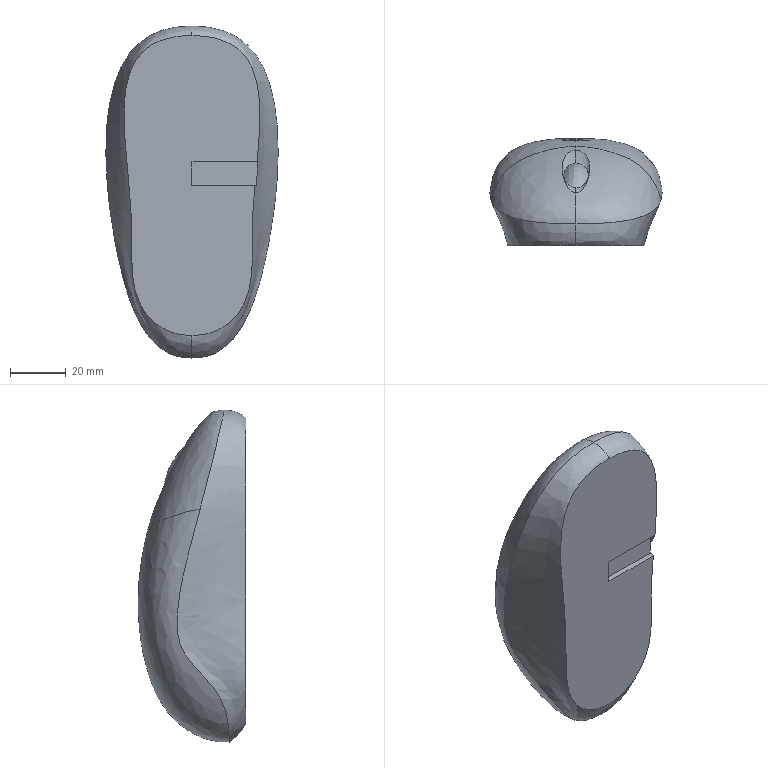Part | STEP file | 11-FG99-mouse-compaq-V3.0-kkkkkk-998.11 | 1 solid | 19 faces | volume 165697 mm3 | spline 13 | plane 6